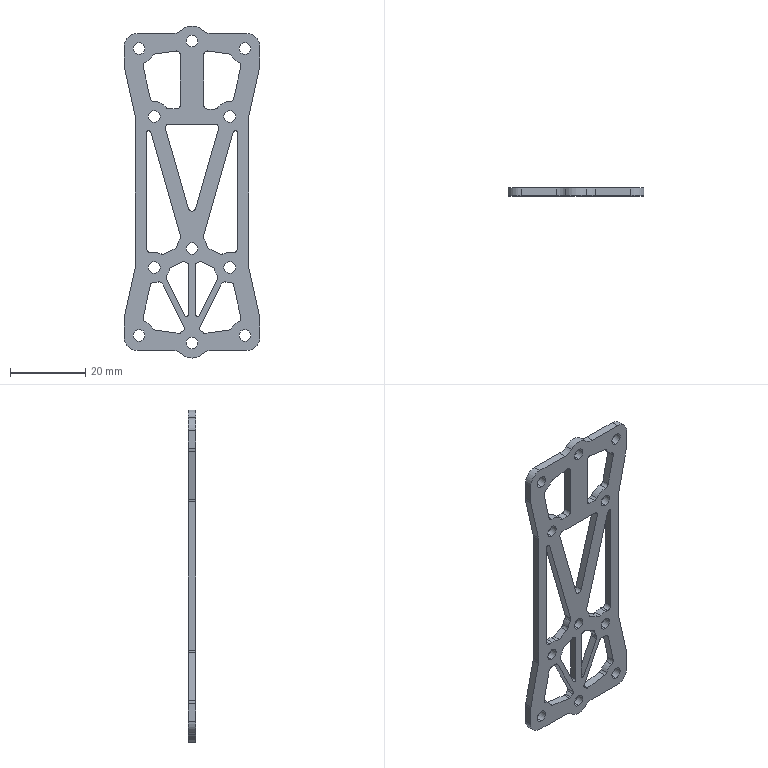Part | SolidWorks | features Fillet 3, Extrusion 1, ICE 1 | 1 solid | 171 faces | box 36 x 2 x 88 mm | volume 3130 mm3 | cylinder 126 | plane 45 | commonest cylinder face diameters 2 x41 8 x27 3.1 x22 1 x20 7 x16